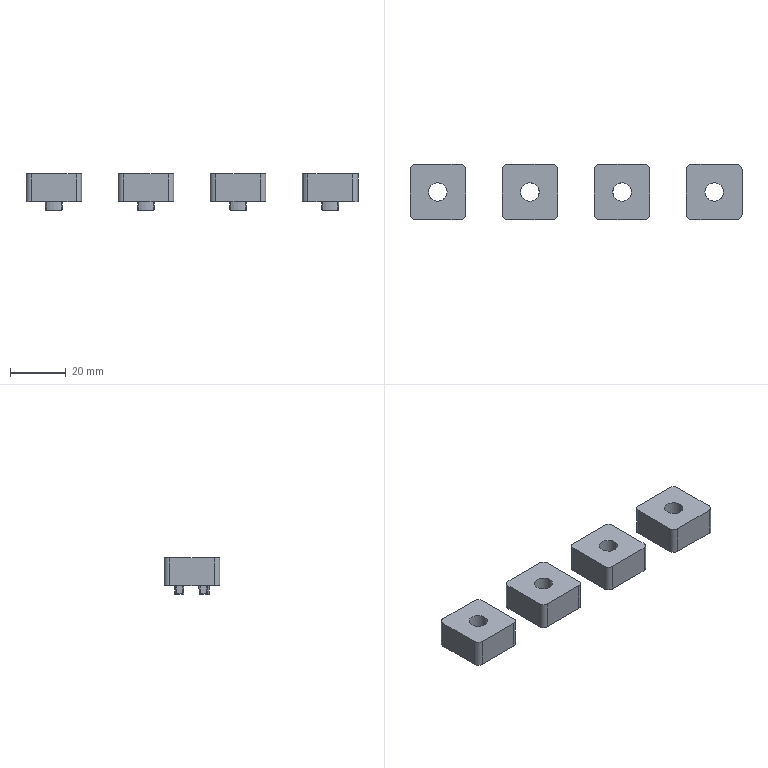NC program | NX | posted with a generic post | part box 118.91 x 19.91 x 13 mm
Lines 4009 to 4960 of 17620:
(FLOOR_WALL_1 , TOOL : D6)
N7992 T12 M6
N7994 G54
N7996 G17 G0 G90 X63.955 Y1.212 S9500 M3
N7998 G43 Z30. H12
N8000 Z0.92
N8002 G94 G1 Z-0.58 F1000.
N8004 X62.755 Y0.52
N8006 G3 X62.455 Y0. R0.6
N8008 G1 Y-8. F2500.
N8010 G2 X57.5 Y-12.955 R4.955
N8012 G1 X41.5
N8014 G2 X36.545 Y-8. R4.955
N8016 G1 Y8.
N8018 G2 X41.5 Y12.955 R4.955
N8020 G1 X45.778
N8022 Y9.355
N8024 G3 X45.124 Y9.068 R10.068
N8026 G1 X44.751 Y8.887
N8028 X44.592 Y8.783
N8030 X43.46 Y7.799
N8032 G3 X43.25 Y7.486 R0.72
N8034 G1 X42.72 Y5.917
N8036 G3 X42.682 Y5.687 R0.72
N8038 G1 X42.685 Y2.783
N8040 X42.766 Y1.87
N8042 G3 X42.861 Y1.573 R0.72
N8044 G1 X43.943 Y-0.291
N8046 G3 X44.32 Y-0.606 R0.72
N8048 G1 X44.45 Y-0.653
N8050 X44.411 Y-0.741
N8052 X43.725 Y-2.632
N8054 G3 X43.682 Y-2.878 R0.72
N8056 G1 Y-6.018
N8058 G3 X43.714 Y-6.231 R0.72
N8060 G1 X44.153 Y-7.65
N8062 G3 X44.321 Y-7.935 R0.72
N8064 G1 X45.313 Y-8.97
N8066 G3 X45.504 Y-9.112 R0.72
N8068 G1 X45.979 Y-9.355
N8070 X41.5
N8072 G2 X40.145 Y-8. R1.355
N8074 G1 Y8.
N8076 G2 X41.5 Y9.355 R1.355
N8078 G1 X45.778
N8080 Y12.955
N8082 X57.5
N8084 G2 X62.455 Y8. R4.955
N8086 G1 Y0.
N8088 X58.855
N8090 Y-8.
N8092 G2 X57.5 Y-9.355 R1.355
N8094 G1 X53.022
N8096 X54.029 Y-8.717
N8098 G3 X54.26 Y-8.481 R0.72
N8100 G1 X55.001 Y-7.255
N8102 G3 X55.089 Y-7.031 R0.72
N8104 G1 X55.303 Y-6.022
N8106 X55.318 Y-5.874
N8108 X55.317 Y-3.292
N8110 X55.272 Y-2.508
N8112 G3 X55.197 Y-2.228 R0.72
N8114 G1 X54.38 Y-0.593
N8116 X55.274 Y-0.074
N8118 G3 X55.589 Y0.303 R0.72
N8120 G1 X56.275 Y2.194
N8122 G3 X56.318 Y2.439 R0.72
N8124 G1 Y5.59
N8126 X56.293 Y5.778
N8128 X55.902 Y7.222
N8130 G3 X55.712 Y7.547 R0.72
N8132 G1 X54.529 Y8.71
N8134 G3 X54.337 Y8.845 R0.72
N8136 G1 X53.876 Y9.068
N8138 G3 X53.222 Y9.355 R10.068
N8140 G1 X52.956 Y8.686
N8142 G2 X53.563 Y8.419 R9.348
N8144 G1 X54.024 Y8.197
N8146 X55.207 Y7.034
N8148 X55.598 Y5.59
N8150 Y2.439
N8152 X54.912 Y0.549
N8154 X53.158 Y-0.47
N8156 X53.612 Y-0.668
N8158 X54.553 Y-2.55
N8160 X54.598 Y-3.334
N8162 Y-5.874
N8164 X54.385 Y-6.883
N8166 X53.644 Y-8.109
N8168 X52.39 Y-8.903
N8170 X51.937 Y-9.025
N8172 G2 X47.063 Y-9.025 R9.348
N8174 G1 X46.749 Y-8.94
N8176 X45.832 Y-8.471
N8178 X44.841 Y-7.437
N8180 X44.402 Y-6.018
N8182 Y-2.878
N8184 X45.088 Y-0.987
N8186 X46.008 Y-0.453
N8188 X44.566 Y0.071
N8190 X43.483 Y1.934
N8192 X43.402 Y2.847
N8194 Y5.687
N8196 X43.932 Y7.255
N8198 X45.064 Y8.239
N8200 X45.437 Y8.419
N8202 G2 X52.956 Y8.686 R9.348
N8204 G1 X53.222 Y9.355
N8206 X57.5
N8208 G2 X58.855 Y8. R1.355
N8210 G1 Y0.
N8212 G3 X59.155 Y-0.52 R0.6
N8214 G1 Z0.92
N8216 G0 X63.955 Y1.212 Z0.34
N8218 G1 Z-1.16 F1000.
N8220 X62.755 Y0.52
N8222 G3 X62.455 Y0. R0.6
N8224 G1 Y-8. F2500.
N8226 G2 X57.5 Y-12.955 R4.955
N8228 G1 X41.5
N8230 G2 X36.545 Y-8. R4.955
N8232 G1 Y8.
N8234 G2 X41.5 Y12.955 R4.955
N8236 G1 X45.778
N8238 Y9.355
N8240 G3 X45.124 Y9.068 R10.068
N8242 G1 X44.751 Y8.887
N8244 X44.592 Y8.783
N8246 X43.46 Y7.799
N8248 G3 X43.25 Y7.486 R0.72
N8250 G1 X42.72 Y5.917
N8252 G3 X42.682 Y5.687 R0.72
N8254 G1 X42.685 Y2.783
N8256 X42.766 Y1.87
N8258 G3 X42.861 Y1.573 R0.72
N8260 G1 X43.943 Y-0.291
N8262 G3 X44.32 Y-0.606 R0.72
N8264 G1 X44.45 Y-0.653
N8266 X44.411 Y-0.741
N8268 X43.725 Y-2.632
N8270 G3 X43.682 Y-2.878 R0.72
N8272 G1 Y-6.018
N8274 G3 X43.714 Y-6.231 R0.72
N8276 G1 X44.153 Y-7.65
N8278 G3 X44.321 Y-7.935 R0.72
N8280 G1 X45.313 Y-8.97
N8282 G3 X45.504 Y-9.112 R0.72
N8284 G1 X45.979 Y-9.355
N8286 X41.5
N8288 G2 X40.145 Y-8. R1.355
N8290 G1 Y8.
N8292 G2 X41.5 Y9.355 R1.355
N8294 G1 X45.778
N8296 Y12.955
N8298 X57.5
N8300 G2 X62.455 Y8. R4.955
N8302 G1 Y0.
N8304 X58.855
N8306 Y-8.
N8308 G2 X57.5 Y-9.355 R1.355
N8310 G1 X53.022
N8312 X54.029 Y-8.717
N8314 G3 X54.26 Y-8.481 R0.72
N8316 G1 X55.001 Y-7.255
N8318 G3 X55.089 Y-7.031 R0.72
N8320 G1 X55.303 Y-6.022
N8322 X55.318 Y-5.874
N8324 X55.317 Y-3.292
N8326 X55.272 Y-2.508
N8328 G3 X55.197 Y-2.228 R0.72
N8330 G1 X54.38 Y-0.593
N8332 X55.274 Y-0.074
N8334 G3 X55.589 Y0.303 R0.72
N8336 G1 X56.275 Y2.194
N8338 G3 X56.318 Y2.439 R0.72
N8340 G1 Y5.59
N8342 X56.293 Y5.778
N8344 X55.902 Y7.222
N8346 G3 X55.712 Y7.547 R0.72
N8348 G1 X54.529 Y8.71
N8350 G3 X54.337 Y8.845 R0.72
N8352 G1 X53.876 Y9.068
N8354 G3 X53.222 Y9.355 R10.068
N8356 G1 X52.956 Y8.686
N8358 G2 X53.563 Y8.419 R9.348
N8360 G1 X54.024 Y8.197
N8362 X55.207 Y7.034
N8364 X55.598 Y5.59
N8366 Y2.439
N8368 X54.912 Y0.549
N8370 X53.158 Y-0.47
N8372 X53.612 Y-0.668
N8374 X54.553 Y-2.55
N8376 X54.598 Y-3.334
N8378 Y-5.874
N8380 X54.385 Y-6.883
N8382 X53.644 Y-8.109
N8384 X52.39 Y-8.903
N8386 X51.937 Y-9.025
N8388 G2 X47.063 Y-9.025 R9.348
N8390 G1 X46.749 Y-8.94
N8392 X45.832 Y-8.471
N8394 X44.841 Y-7.437
N8396 X44.402 Y-6.018
N8398 Y-2.878
N8400 X45.088 Y-0.987
N8402 X46.008 Y-0.453
N8404 X44.566 Y0.071
N8406 X43.483 Y1.934
N8408 X43.402 Y2.847
N8410 Y5.687
N8412 X43.932 Y7.255
N8414 X45.064 Y8.239
N8416 X45.437 Y8.419
N8418 G2 X52.956 Y8.686 R9.348
N8420 G1 X53.222 Y9.355
N8422 X57.5
N8424 G2 X58.855 Y8. R1.355
N8426 G1 Y0.
N8428 G3 X59.155 Y-0.52 R0.6
N8430 G1 Z0.34
N8432 G0 X63.955 Y1.212 Z-0.24
N8434 G1 Z-1.74 F1000.
N8436 X62.755 Y0.52
N8438 G3 X62.455 Y0. R0.6
N8440 G1 Y-8. F2500.
N8442 G2 X57.5 Y-12.955 R4.955
N8444 G1 X41.5
N8446 G2 X36.545 Y-8. R4.955
N8448 G1 Y8.
N8450 G2 X41.5 Y12.955 R4.955
N8452 G1 X45.778
N8454 Y9.355
N8456 G3 X45.124 Y9.068 R10.068
N8458 G1 X44.751 Y8.887
N8460 X44.592 Y8.783
N8462 X43.46 Y7.799
N8464 G3 X43.25 Y7.486 R0.72
N8466 G1 X42.72 Y5.917
N8468 G3 X42.682 Y5.687 R0.72
N8470 G1 X42.685 Y2.783
N8472 X42.766 Y1.87
N8474 G3 X42.861 Y1.573 R0.72
N8476 G1 X43.943 Y-0.291
N8478 G3 X44.32 Y-0.606 R0.72
N8480 G1 X44.45 Y-0.653
N8482 X44.411 Y-0.741
N8484 X43.725 Y-2.632
N8486 G3 X43.682 Y-2.878 R0.72
N8488 G1 Y-6.018
N8490 G3 X43.714 Y-6.231 R0.72
N8492 G1 X44.153 Y-7.65
N8494 G3 X44.321 Y-7.935 R0.72
N8496 G1 X45.313 Y-8.97
N8498 G3 X45.504 Y-9.112 R0.72
N8500 G1 X45.979 Y-9.355
N8502 X41.5
N8504 G2 X40.145 Y-8. R1.355
N8506 G1 Y8.
N8508 G2 X41.5 Y9.355 R1.355
N8510 G1 X45.778
N8512 Y12.955
N8514 X57.5
N8516 G2 X62.455 Y8. R4.955
N8518 G1 Y0.
N8520 X58.855
N8522 Y-8.
N8524 G2 X57.5 Y-9.355 R1.355
N8526 G1 X53.022
N8528 X54.029 Y-8.717
N8530 G3 X54.26 Y-8.481 R0.72
N8532 G1 X55.001 Y-7.255
N8534 G3 X55.089 Y-7.031 R0.72
N8536 G1 X55.303 Y-6.022
N8538 X55.318 Y-5.874
N8540 X55.317 Y-3.292
N8542 X55.272 Y-2.508
N8544 G3 X55.197 Y-2.228 R0.72
N8546 G1 X54.38 Y-0.593
N8548 X55.274 Y-0.074
N8550 G3 X55.589 Y0.303 R0.72
N8552 G1 X56.275 Y2.194
N8554 G3 X56.318 Y2.439 R0.72
N8556 G1 Y5.59
N8558 X56.293 Y5.778
N8560 X55.902 Y7.222
N8562 G3 X55.712 Y7.547 R0.72
N8564 G1 X54.529 Y8.71
N8566 G3 X54.337 Y8.845 R0.72
N8568 G1 X53.876 Y9.068
N8570 G3 X53.222 Y9.355 R10.068
N8572 G1 X52.956 Y8.686
N8574 G2 X53.563 Y8.419 R9.348
N8576 G1 X54.024 Y8.197
N8578 X55.207 Y7.034
N8580 X55.598 Y5.59
N8582 Y2.439
N8584 X54.912 Y0.549
N8586 X53.158 Y-0.47
N8588 X53.612 Y-0.668
N8590 X54.553 Y-2.55
N8592 X54.598 Y-3.334
N8594 Y-5.874
N8596 X54.385 Y-6.883
N8598 X53.644 Y-8.109
N8600 X52.39 Y-8.903
N8602 X51.937 Y-9.025
N8604 G2 X47.063 Y-9.025 R9.348
N8606 G1 X46.749 Y-8.94
N8608 X45.832 Y-8.471
N8610 X44.841 Y-7.437
N8612 X44.402 Y-6.018
N8614 Y-2.878
N8616 X45.088 Y-0.987
N8618 X46.008 Y-0.453
N8620 X44.566 Y0.071
N8622 X43.483 Y1.934
N8624 X43.402 Y2.847
N8626 Y5.687
N8628 X43.932 Y7.255
N8630 X45.064 Y8.239
N8632 X45.437 Y8.419
N8634 G2 X52.956 Y8.686 R9.348
N8636 G1 X53.222 Y9.355
N8638 X57.5
N8640 G2 X58.855 Y8. R1.355
N8642 G1 Y0.
N8644 G3 X59.155 Y-0.52 R0.6
N8646 G1 Z-0.24
N8648 G0 X63.955 Y1.212 Z-0.82
N8650 G1 Z-2.32 F1000.
N8652 X62.755 Y0.52
N8654 G3 X62.455 Y0. R0.6
N8656 G1 Y-8. F2500.
N8658 G2 X57.5 Y-12.955 R4.955
N8660 G1 X41.5
N8662 G2 X36.545 Y-8. R4.955
N8664 G1 Y8.
N8666 G2 X41.5 Y12.955 R4.955
N8668 G1 X45.778
N8670 Y9.355
N8672 G3 X45.124 Y9.068 R10.068
N8674 G1 X44.751 Y8.887
N8676 X44.592 Y8.783
N8678 X43.46 Y7.799
N8680 G3 X43.25 Y7.486 R0.72
N8682 G1 X42.72 Y5.917
N8684 G3 X42.682 Y5.687 R0.72
N8686 G1 X42.685 Y2.783
N8688 X42.766 Y1.87
N8690 G3 X42.861 Y1.573 R0.72
N8692 G1 X43.943 Y-0.291
N8694 G3 X44.32 Y-0.606 R0.72
N8696 G1 X44.45 Y-0.653
N8698 X44.411 Y-0.741
N8700 X43.725 Y-2.632
N8702 G3 X43.682 Y-2.878 R0.72
N8704 G1 Y-6.018
N8706 G3 X43.714 Y-6.231 R0.72
N8708 G1 X44.153 Y-7.65
N8710 G3 X44.321 Y-7.935 R0.72
N8712 G1 X45.313 Y-8.97
N8714 G3 X45.504 Y-9.112 R0.72
N8716 G1 X45.979 Y-9.355
N8718 X41.5
N8720 G2 X40.145 Y-8. R1.355
N8722 G1 Y8.
N8724 G2 X41.5 Y9.355 R1.355
N8726 G1 X45.778
N8728 Y12.955
N8730 X57.5
N8732 G2 X62.455 Y8. R4.955
N8734 G1 Y0.
N8736 X58.855
N8738 Y-8.
N8740 G2 X57.5 Y-9.355 R1.355
N8742 G1 X53.022
N8744 X54.029 Y-8.717
N8746 G3 X54.26 Y-8.481 R0.72
N8748 G1 X55.001 Y-7.255
N8750 G3 X55.089 Y-7.031 R0.72
N8752 G1 X55.303 Y-6.022
N8754 X55.318 Y-5.874
N8756 X55.317 Y-3.292
N8758 X55.272 Y-2.508
N8760 G3 X55.197 Y-2.228 R0.72
N8762 G1 X54.38 Y-0.593
N8764 X55.274 Y-0.074
N8766 G3 X55.589 Y0.303 R0.72
N8768 G1 X56.275 Y2.194
N8770 G3 X56.318 Y2.439 R0.72
N8772 G1 Y5.59
N8774 X56.293 Y5.778
N8776 X55.902 Y7.222
N8778 G3 X55.712 Y7.547 R0.72
N8780 G1 X54.529 Y8.71
N8782 G3 X54.337 Y8.845 R0.72
N8784 G1 X53.876 Y9.068
N8786 G3 X53.222 Y9.355 R10.068
N8788 G1 X52.956 Y8.686
N8790 G2 X53.563 Y8.419 R9.348
N8792 G1 X54.024 Y8.197
N8794 X55.207 Y7.034
N8796 X55.598 Y5.59
N8798 Y2.439
N8800 X54.912 Y0.549
N8802 X53.158 Y-0.47
N8804 X53.612 Y-0.668
N8806 X54.553 Y-2.55
N8808 X54.598 Y-3.334
N8810 Y-5.874
N8812 X54.385 Y-6.883
N8814 X53.644 Y-8.109
N8816 X52.39 Y-8.903
N8818 X51.937 Y-9.025
N8820 G2 X47.063 Y-9.025 R9.348
N8822 G1 X46.749 Y-8.94
N8824 X45.832 Y-8.471
N8826 X44.841 Y-7.437
N8828 X44.402 Y-6.018
N8830 Y-2.878
N8832 X45.088 Y-0.987
N8834 X46.008 Y-0.453
N8836 X44.566 Y0.071
N8838 X43.483 Y1.934
N8840 X43.402 Y2.847
N8842 Y5.687
N8844 X43.932 Y7.255
N8846 X45.064 Y8.239
N8848 X45.437 Y8.419
N8850 G2 X52.956 Y8.686 R9.348
N8852 G1 X53.222 Y9.355
N8854 X57.5
N8856 G2 X58.855 Y8. R1.355
N8858 G1 Y0.
N8860 G3 X59.155 Y-0.52 R0.6
N8862 G1 Z-0.82
N8864 G0 X63.955 Y1.212 Z-1.4
N8866 G1 Z-2.9 F1000.
N8868 X62.755 Y0.52
N8870 G3 X62.455 Y0. R0.6
N8872 G1 Y-8. F2500.
N8874 G2 X57.5 Y-12.955 R4.955
N8876 G1 X41.5
N8878 G2 X36.545 Y-8. R4.955
N8880 G1 Y8.
N8882 G2 X41.5 Y12.955 R4.955
N8884 G1 X45.778
N8886 Y9.355
N8888 G3 X45.124 Y9.068 R10.068
N8890 G1 X44.751 Y8.887
N8892 X44.592 Y8.783
N8894 X43.46 Y7.799
N8896 G3 X43.25 Y7.486 R0.72
N8898 G1 X42.72 Y5.917
N8900 G3 X42.682 Y5.687 R0.72
N8902 G1 X42.685 Y2.783
N8904 X42.766 Y1.87
N8906 G3 X42.861 Y1.573 R0.72
N8908 G1 X43.943 Y-0.291
N8910 G3 X44.32 Y-0.606 R0.72
N8912 G1 X44.45 Y-0.653
N8914 X44.411 Y-0.741
N8916 X43.725 Y-2.632
N8918 G3 X43.682 Y-2.878 R0.72
N8920 G1 Y-6.018
N8922 G3 X43.714 Y-6.231 R0.72
N8924 G1 X44.153 Y-7.65
N8926 G3 X44.321 Y-7.935 R0.72
N8928 G1 X45.313 Y-8.97
N8930 G3 X45.504 Y-9.112 R0.72
N8932 G1 X45.979 Y-9.355
N8934 X41.5
N8936 G2 X40.145 Y-8. R1.355
N8938 G1 Y8.
N8940 G2 X41.5 Y9.355 R1.355
N8942 G1 X45.778
N8944 Y12.955
N8946 X57.5
N8948 G2 X62.455 Y8. R4.955
N8950 G1 Y0.
N8952 X58.855
N8954 Y-8.
N8956 G2 X57.5 Y-9.355 R1.355
N8958 G1 X53.022
N8960 X54.029 Y-8.717
N8962 G3 X54.26 Y-8.481 R0.72
N8964 G1 X55.001 Y-7.255
N8966 G3 X55.089 Y-7.031 R0.72
N8968 G1 X55.303 Y-6.022
N8970 X55.318 Y-5.874
N8972 X55.317 Y-3.292
N8974 X55.272 Y-2.508
N8976 G3 X55.197 Y-2.228 R0.72
N8978 G1 X54.38 Y-0.593
N8980 X55.274 Y-0.074
N8982 G3 X55.589 Y0.303 R0.72
N8984 G1 X56.275 Y2.194
N8986 G3 X56.318 Y2.439 R0.72
N8988 G1 Y5.59
N8990 X56.293 Y5.778
N8992 X55.902 Y7.222
N8994 G3 X55.712 Y7.547 R0.72
N8996 G1 X54.529 Y8.71
N8998 G3 X54.337 Y8.845 R0.72
N9000 G1 X53.876 Y9.068
N9002 G3 X53.222 Y9.355 R10.068
N9004 G1 X52.956 Y8.686
N9006 G2 X53.563 Y8.419 R9.348
N9008 G1 X54.024 Y8.197
N9010 X55.207 Y7.034
N9012 X55.598 Y5.59
N9014 Y2.439
N9016 X54.912 Y0.549
N9018 X53.158 Y-0.47
N9020 X53.612 Y-0.668
N9022 X54.553 Y-2.55
N9024 X54.598 Y-3.334
N9026 Y-5.874
N9028 X54.385 Y-6.883
N9030 X53.644 Y-8.109
N9032 X52.39 Y-8.903
N9034 X51.937 Y-9.025
N9036 G2 X47.063 Y-9.025 R9.348
N9038 G1 X46.749 Y-8.94
N9040 X45.832 Y-8.471
N9042 X44.841 Y-7.437
N9044 X44.402 Y-6.018
N9046 Y-2.878
N9048 X45.088 Y-0.987
N9050 X46.008 Y-0.453
N9052 X44.566 Y0.071
N9054 X43.483 Y1.934
N9056 X43.402 Y2.847
N9058 Y5.687
N9060 X43.932 Y7.255
N9062 X45.064 Y8.239
N9064 X45.437 Y8.419
N9066 G2 X52.956 Y8.686 R9.348
N9068 G1 X53.222 Y9.355
N9070 X57.5
N9072 G2 X58.855 Y8. R1.355
N9074 G1 Y0.
N9076 G3 X59.155 Y-0.52 R0.6
N9078 G1 Z-1.4
N9080 G0 Z30.
N9082 X49.153 Y-0.044
N9084 Z1.5
N9086 G1 X49.148 Y-0.042 Z1.499 F1000.
N9088 X49.2 Y0.003 Z1.48
N9090 X49.148 Y-0.042 Z1.462
N9092 X49.209 Y-0.074 Z1.443
N9094 X49.148 Y-0.042 Z1.425
N9096 X49.2 Y0.003 Z1.407
N9098 X49.148 Y-0.042 Z1.388
N9100 X49.209 Y-0.074 Z1.37
N9102 X49.148 Y-0.042 Z1.352
N9104 X49.2 Y0.003 Z1.333
N9106 X49.148 Y-0.042 Z1.315
N9108 X49.209 Y-0.074 Z1.296
N9110 X49.148 Y-0.042 Z1.278
N9112 X49.2 Y0.003 Z1.26
N9114 X49.148 Y-0.042 Z1.241
N9116 X49.209 Y-0.074 Z1.223
N9118 X49.148 Y-0.042 Z1.204
N9120 X49.2 Y0.003 Z1.186
N9122 X49.148 Y-0.042 Z1.168
N9124 X49.209 Y-0.074 Z1.149
N9126 X49.148 Y-0.042 Z1.131
N9128 X49.2 Y0.003 Z1.112
N9130 X49.148 Y-0.042 Z1.094
N9132 X49.209 Y-0.074 Z1.076
N9134 X49.148 Y-0.042 Z1.057
N9136 X49.2 Y0.003 Z1.039
N9138 X49.148 Y-0.042 Z1.02
N9140 X49.209 Y-0.074 Z1.002
N9142 X49.148 Y-0.042 Z0.984
N9144 X49.2 Y0.003 Z0.965
N9146 X49.148 Y-0.042 Z0.947
N9148 X49.209 Y-0.074 Z0.928
N9150 X49.148 Y-0.042 Z0.91
N9152 X49.2 Y0.003 Z0.892
N9154 X49.148 Y-0.042 Z0.873
N9156 X49.209 Y-0.074 Z0.855
N9158 X49.148 Y-0.042 Z0.836
N9160 X49.2 Y0.003 Z0.818
N9162 X49.148 Y-0.042 Z0.8
N9164 X49.209 Y-0.074 Z0.781
N9166 X49.148 Y-0.042 Z0.763
N9168 X49.2 Y0.003 Z0.744
N9170 X49.148 Y-0.042 Z0.726
N9172 X49.209 Y-0.074 Z0.708
N9174 X49.148 Y-0.042 Z0.689
N9176 X49.2 Y0.003 Z0.671
N9178 X49.148 Y-0.042 Z0.652
N9180 X49.209 Y-0.074 Z0.634
N9182 X49.148 Y-0.042 Z0.616
N9184 X49.2 Y0.003 Z0.597
N9186 X49.148 Y-0.042 Z0.579
N9188 X49.209 Y-0.074 Z0.561
N9190 X49.148 Y-0.042 Z0.542
N9192 X49.2 Y0.003 Z0.524
N9194 X49.148 Y-0.042 Z0.505
N9196 X49.209 Y-0.074 Z0.487
N9198 X49.148 Y-0.042 Z0.469
N9200 X49.2 Y0.003 Z0.45
N9202 X49.148 Y-0.042 Z0.432
N9204 X49.209 Y-0.074 Z0.413
N9206 X49.148 Y-0.042 Z0.395
N9208 X49.2 Y0.003 Z0.377
N9210 X49.148 Y-0.042 Z0.358
N9212 X49.209 Y-0.074 Z0.34
N9214 X49.148 Y-0.042 Z0.321
N9216 X49.2 Y0.003 Z0.303
N9218 X49.148 Y-0.042 Z0.285
N9220 X49.209 Y-0.074 Z0.266
N9222 X49.148 Y-0.042 Z0.248
N9224 X49.2 Y0.003 Z0.229
N9226 X49.148 Y-0.042 Z0.211
N9228 X49.209 Y-0.074 Z0.193
N9230 X49.148 Y-0.042 Z0.174
N9232 X49.2 Y0.003 Z0.156
N9234 X49.148 Y-0.042 Z0.137
N9236 X49.209 Y-0.074 Z0.119
N9238 X49.148 Y-0.042 Z0.101
N9240 X49.2 Y0.003 Z0.082
N9242 X49.148 Y-0.042 Z0.064
N9244 X49.209 Y-0.074 Z0.045
N9246 X49.148 Y-0.042 Z0.027
N9248 X49.2 Y0.003 Z0.009
N9250 X49.148 Y-0.042 Z-0.01
N9252 X49.209 Y-0.074 Z-0.028
N9254 X49.148 Y-0.042 Z-0.047
N9256 X49.2 Y0.003 Z-0.065
N9258 X49.148 Y-0.042 Z-0.083
N9260 X49.209 Y-0.074 Z-0.102
N9262 X49.148 Y-0.042 Z-0.12
N9264 X49.2 Y0.003 Z-0.139
N9266 X49.148 Y-0.042 Z-0.157
N9268 X49.209 Y-0.074 Z-0.175
N9270 X49.148 Y-0.042 Z-0.194
N9272 X49.2 Y0.003 Z-0.212
N9274 X49.148 Y-0.042 Z-0.23
N9276 X49.209 Y-0.074 Z-0.249
N9278 X49.148 Y-0.042 Z-0.267
N9280 X49.2 Y0.003 Z-0.286
N9282 X49.148 Y-0.042 Z-0.304
N9284 X49.209 Y-0.074 Z-0.322
N9286 X49.148 Y-0.042 Z-0.341
N9288 X49.2 Y0.003 Z-0.359
N9290 X49.148 Y-0.042 Z-0.378
N9292 X49.209 Y-0.074 Z-0.396
N9294 X49.148 Y-0.042 Z-0.414
N9296 X49.2 Y0.003 Z-0.433
N9298 X49.148 Y-0.042 Z-0.451
N9300 X49.209 Y-0.074 Z-0.47
N9302 X49.148 Y-0.042 Z-0.488
N9304 X49.2 Y0.003 Z-0.506
N9306 X49.148 Y-0.042 Z-0.525
N9308 X49.209 Y-0.074 Z-0.543
N9310 X49.148 Y-0.042 Z-0.562
N9312 X49.2 Y0.003 Z-0.58
N9314 X49.148 Y-0.042 F2500.
N9316 X49.209 Y-0.074
N9318 Z0.92
N9320 G0 X49.153 Y-0.044
N9322 G1 X49.148 Y-0.042 Z0.919 F1000.
N9324 X49.2 Y0.003 Z0.9
N9326 X49.148 Y-0.042 Z0.882
N9328 X49.209 Y-0.074 Z0.863
N9330 X49.148 Y-0.042 Z0.845
N9332 X49.2 Y0.003 Z0.827
N9334 X49.148 Y-0.042 Z0.808
N9336 X49.209 Y-0.074 Z0.79
N9338 X49.148 Y-0.042 Z0.772
N9340 X49.2 Y0.003 Z0.753
N9342 X49.148 Y-0.042 Z0.735
N9344 X49.209 Y-0.074 Z0.716
N9346 X49.148 Y-0.042 Z0.698
N9348 X49.2 Y0.003 Z0.68
N9350 X49.148 Y-0.042 Z0.661
N9352 X49.209 Y-0.074 Z0.643
N9354 X49.148 Y-0.042 Z0.624
N9356 X49.2 Y0.003 Z0.606
N9358 X49.148 Y-0.042 Z0.588
N9360 X49.209 Y-0.074 Z0.569
N9362 X49.148 Y-0.042 Z0.551
N9364 X49.2 Y0.003 Z0.532
N9366 X49.148 Y-0.042 Z0.514
N9368 X49.209 Y-0.074 Z0.496
N9370 X49.148 Y-0.042 Z0.477
N9372 X49.2 Y0.003 Z0.459
N9374 X49.148 Y-0.042 Z0.44
N9376 X49.209 Y-0.074 Z0.422
N9378 X49.148 Y-0.042 Z0.404
N9380 X49.2 Y0.003 Z0.385
N9382 X49.148 Y-0.042 Z0.367
N9384 X49.209 Y-0.074 Z0.348
N9386 X49.148 Y-0.042 Z0.33
N9388 X49.2 Y0.003 Z0.312
N9390 X49.148 Y-0.042 Z0.293
N9392 X49.209 Y-0.074 Z0.275
N9394 X49.148 Y-0.042 Z0.256
N9396 X49.2 Y0.003 Z0.238
N9398 X49.148 Y-0.042 Z0.22
N9400 X49.209 Y-0.074 Z0.201
N9402 X49.148 Y-0.042 Z0.183
N9404 X49.2 Y0.003 Z0.164
N9406 X49.148 Y-0.042 Z0.146
N9408 X49.209 Y-0.074 Z0.128
N9410 X49.148 Y-0.042 Z0.109
N9412 X49.2 Y0.003 Z0.091
N9414 X49.148 Y-0.042 Z0.072
N9416 X49.209 Y-0.074 Z0.054
N9418 X49.148 Y-0.042 Z0.036
N9420 X49.2 Y0.003 Z0.017
N9422 X49.148 Y-0.042 Z-0.001
N9424 X49.209 Y-0.074 Z-0.019
N9426 X49.148 Y-0.042 Z-0.038
N9428 X49.2 Y0.003 Z-0.056
N9430 X49.148 Y-0.042 Z-0.075
N9432 X49.209 Y-0.074 Z-0.093
N9434 X49.148 Y-0.042 Z-0.111
N9436 X49.2 Y0.003 Z-0.13
N9438 X49.148 Y-0.042 Z-0.148
N9440 X49.209 Y-0.074 Z-0.167
N9442 X49.148 Y-0.042 Z-0.185
N9444 X49.2 Y0.003 Z-0.203
N9446 X49.148 Y-0.042 Z-0.222
N9448 X49.209 Y-0.074 Z-0.24
N9450 X49.148 Y-0.042 Z-0.259
N9452 X49.2 Y0.003 Z-0.277
N9454 X49.148 Y-0.042 Z-0.295
N9456 X49.209 Y-0.074 Z-0.314
N9458 X49.148 Y-0.042 Z-0.332
N9460 X49.2 Y0.003 Z-0.351
N9462 X49.148 Y-0.042 Z-0.369
N9464 X49.209 Y-0.074 Z-0.387
N9466 X49.148 Y-0.042 Z-0.406
N9468 X49.2 Y0.003 Z-0.424
N9470 X49.148 Y-0.042 Z-0.443
N9472 X49.209 Y-0.074 Z-0.461
N9474 X49.148 Y-0.042 Z-0.479
N9476 X49.2 Y0.003 Z-0.498
N9478 X49.148 Y-0.042 Z-0.516
N9480 X49.209 Y-0.074 Z-0.535
N9482 X49.148 Y-0.042 Z-0.553
N9484 X49.2 Y0.003 Z-0.571
N9486 X49.148 Y-0.042 Z-0.59
N9488 X49.209 Y-0.074 Z-0.608
N9490 X49.148 Y-0.042 Z-0.627
N9492 X49.2 Y0.003 Z-0.645
N9494 X49.148 Y-0.042 Z-0.663
N9496 X49.209 Y-0.074 Z-0.682
N9498 X49.148 Y-0.042 Z-0.7
N9500 X49.2 Y0.003 Z-0.719
N9502 X49.148 Y-0.042 Z-0.737
N9504 X49.209 Y-0.074 Z-0.755
N9506 X49.148 Y-0.042 Z-0.774
N9508 X49.2 Y0.003 Z-0.792
N9510 X49.148 Y-0.042 Z-0.81
N9512 X49.209 Y-0.074 Z-0.829
N9514 X49.148 Y-0.042 Z-0.847
N9516 X49.2 Y0.003 Z-0.866
N9518 X49.148 Y-0.042 Z-0.884
N9520 X49.209 Y-0.074 Z-0.902
N9522 X49.148 Y-0.042 Z-0.921
N9524 X49.2 Y0.003 Z-0.939
N9526 X49.148 Y-0.042 Z-0.958
N9528 X49.209 Y-0.074 Z-0.976
N9530 X49.148 Y-0.042 Z-0.994
N9532 X49.2 Y0.003 Z-1.013
N9534 X49.148 Y-0.042 Z-1.031
N9536 X49.209 Y-0.074 Z-1.05
N9538 X49.148 Y-0.042 Z-1.068
N9540 X49.2 Y0.003 Z-1.086
N9542 X49.148 Y-0.042 Z-1.105
N9544 X49.209 Y-0.074 Z-1.123
N9546 X49.148 Y-0.042 Z-1.142
N9548 X49.2 Y0.003 Z-1.16
N9550 X49.148 Y-0.042 F2500.
N9552 X49.209 Y-0.074
N9554 Z0.34
N9556 G0 X49.153 Y-0.044
N9558 G1 X49.148 Y-0.042 Z0.339 F1000.
N9560 X49.2 Y0.003 Z0.32
N9562 X49.148 Y-0.042 Z0.302
N9564 X49.209 Y-0.074 Z0.283
N9566 X49.148 Y-0.042 Z0.265
N9568 X49.2 Y0.003 Z0.247
N9570 X49.148 Y-0.042 Z0.228
N9572 X49.209 Y-0.074 Z0.21
N9574 X49.148 Y-0.042 Z0.192
N9576 X49.2 Y0.003 Z0.173
N9578 X49.148 Y-0.042 Z0.155
N9580 X49.209 Y-0.074 Z0.136
N9582 X49.148 Y-0.042 Z0.118
N9584 X49.2 Y0.003 Z0.1
N9586 X49.148 Y-0.042 Z0.081
N9588 X49.209 Y-0.074 Z0.063
N9590 X49.148 Y-0.042 Z0.044
N9592 X49.2 Y0.003 Z0.026
N9594 X49.148 Y-0.042 Z0.008
N9596 X49.209 Y-0.074 Z-0.011
N9598 X49.148 Y-0.042 Z-0.029
N9600 X49.2 Y0.003 Z-0.048
N9602 X49.148 Y-0.042 Z-0.066
N9604 X49.209 Y-0.074 Z-0.084
N9606 X49.148 Y-0.042 Z-0.103
N9608 X49.2 Y0.003 Z-0.121
N9610 X49.148 Y-0.042 Z-0.14
N9612 X49.209 Y-0.074 Z-0.158
N9614 X49.148 Y-0.042 Z-0.176
N9616 X49.2 Y0.003 Z-0.195
N9618 X49.148 Y-0.042 Z-0.213
N9620 X49.209 Y-0.074 Z-0.232
N9622 X49.148 Y-0.042 Z-0.25
N9624 X49.2 Y0.003 Z-0.268
N9626 X49.148 Y-0.042 Z-0.287
N9628 X49.209 Y-0.074 Z-0.305
N9630 X49.148 Y-0.042 Z-0.324
N9632 X49.2 Y0.003 Z-0.342
N9634 X49.148 Y-0.042 Z-0.36
N9636 X49.209 Y-0.074 Z-0.379
N9638 X49.148 Y-0.042 Z-0.397
N9640 X49.2 Y0.003 Z-0.416
N9642 X49.148 Y-0.042 Z-0.434
N9644 X49.209 Y-0.074 Z-0.452
N9646 X49.148 Y-0.042 Z-0.471
N9648 X49.2 Y0.003 Z-0.489
N9650 X49.148 Y-0.042 Z-0.508
N9652 X49.209 Y-0.074 Z-0.526
N9654 X49.148 Y-0.042 Z-0.544
N9656 X49.2 Y0.003 Z-0.563
N9658 X49.148 Y-0.042 Z-0.581
N9660 X49.209 Y-0.074 Z-0.599
N9662 X49.148 Y-0.042 Z-0.618
N9664 X49.2 Y0.003 Z-0.636
N9666 X49.148 Y-0.042 Z-0.655
N9668 X49.209 Y-0.074 Z-0.673
N9670 X49.148 Y-0.042 Z-0.691
N9672 X49.2 Y0.003 Z-0.71
N9674 X49.148 Y-0.042 Z-0.728
N9676 X49.209 Y-0.074 Z-0.747
N9678 X49.148 Y-0.042 Z-0.765
N9680 X49.2 Y0.003 Z-0.783
N9682 X49.148 Y-0.042 Z-0.802
N9684 X49.209 Y-0.074 Z-0.82
N9686 X49.148 Y-0.042 Z-0.839
N9688 X49.2 Y0.003 Z-0.857
N9690 X49.148 Y-0.042 Z-0.875
N9692 X49.209 Y-0.074 Z-0.894
N9694 X49.148 Y-0.042 Z-0.912
N9696 X49.2 Y0.003 Z-0.931
N9698 X49.148 Y-0.042 Z-0.949
N9700 X49.209 Y-0.074 Z-0.967
N9702 X49.148 Y-0.042 Z-0.986
N9704 X49.2 Y0.003 Z-1.004
N9706 X49.148 Y-0.042 Z-1.023
N9708 X49.209 Y-0.074 Z-1.041
N9710 X49.148 Y-0.042 Z-1.059
N9712 X49.2 Y0.003 Z-1.078
N9714 X49.148 Y-0.042 Z-1.096
N9716 X49.209 Y-0.074 Z-1.115
N9718 X49.148 Y-0.042 Z-1.133
N9720 X49.2 Y0.003 Z-1.151
N9722 X49.148 Y-0.042 Z-1.17
N9724 X49.209 Y-0.074 Z-1.188
N9726 X49.148 Y-0.042 Z-1.207
N9728 X49.2 Y0.003 Z-1.225
N9730 X49.148 Y-0.042 Z-1.243
N9732 X49.209 Y-0.074 Z-1.262
N9734 X49.148 Y-0.042 Z-1.28
N9736 X49.2 Y0.003 Z-1.299
N9738 X49.148 Y-0.042 Z-1.317
N9740 X49.209 Y-0.074 Z-1.335
N9742 X49.148 Y-0.042 Z-1.354
N9744 X49.2 Y0.003 Z-1.372
N9746 X49.148 Y-0.042 Z-1.39
N9748 X49.209 Y-0.074 Z-1.409
N9750 X49.148 Y-0.042 Z-1.427
N9752 X49.2 Y0.003 Z-1.446
N9754 X49.148 Y-0.042 Z-1.464
N9756 X49.209 Y-0.074 Z-1.482
N9758 X49.148 Y-0.042 Z-1.501
N9760 X49.2 Y0.003 Z-1.519
N9762 X49.148 Y-0.042 Z-1.538
N9764 X49.209 Y-0.074 Z-1.556
N9766 X49.148 Y-0.042 Z-1.574
N9768 X49.2 Y0.003 Z-1.593
N9770 X49.148 Y-0.042 Z-1.611
N9772 X49.209 Y-0.074 Z-1.63
N9774 X49.148 Y-0.042 Z-1.648
N9776 X49.2 Y0.003 Z-1.666
N9778 X49.148 Y-0.042 Z-1.685
N9780 X49.209 Y-0.074 Z-1.703
N9782 X49.148 Y-0.042 Z-1.722
N9784 X49.2 Y0.003 Z-1.74
N9786 X49.148 Y-0.042 F2500.
N9788 X49.209 Y-0.074
N9790 Z-0.24
N9792 G0 X49.153 Y-0.044
N9794 G1 X49.148 Y-0.042 Z-0.241 F1000.
N9796 X49.2 Y0.003 Z-0.26
N9798 X49.148 Y-0.042 Z-0.278
N9800 X49.209 Y-0.074 Z-0.297
N9802 X49.148 Y-0.042 Z-0.315
N9804 X49.2 Y0.003 Z-0.333
N9806 X49.148 Y-0.042 Z-0.352
N9808 X49.209 Y-0.074 Z-0.37
N9810 X49.148 Y-0.042 Z-0.388
N9812 X49.2 Y0.003 Z-0.407
N9814 X49.148 Y-0.042 Z-0.425
N9816 X49.209 Y-0.074 Z-0.444
N9818 X49.148 Y-0.042 Z-0.462
N9820 X49.2 Y0.003 Z-0.48
N9822 X49.148 Y-0.042 Z-0.499
N9824 X49.209 Y-0.074 Z-0.517
N9826 X49.148 Y-0.042 Z-0.536
N9828 X49.2 Y0.003 Z-0.554
N9830 X49.148 Y-0.042 Z-0.572
N9832 X49.209 Y-0.074 Z-0.591
N9834 X49.148 Y-0.042 Z-0.609
N9836 X49.2 Y0.003 Z-0.628
N9838 X49.148 Y-0.042 Z-0.646
N9840 X49.209 Y-0.074 Z-0.664
N9842 X49.148 Y-0.042 Z-0.683
N9844 X49.2 Y0.003 Z-0.701
N9846 X49.148 Y-0.042 Z-0.72
N9848 X49.209 Y-0.074 Z-0.738
N9850 X49.148 Y-0.042 Z-0.756
N9852 X49.2 Y0.003 Z-0.775
N9854 X49.148 Y-0.042 Z-0.793
N9856 X49.209 Y-0.074 Z-0.812
N9858 X49.148 Y-0.042 Z-0.83
N9860 X49.2 Y0.003 Z-0.848
N9862 X49.148 Y-0.042 Z-0.867
N9864 X49.209 Y-0.074 Z-0.885
N9866 X49.148 Y-0.042 Z-0.904
N9868 X49.2 Y0.003 Z-0.922
N9870 X49.148 Y-0.042 Z-0.94
N9872 X49.209 Y-0.074 Z-0.959
N9874 X49.148 Y-0.042 Z-0.977
N9876 X49.2 Y0.003 Z-0.996
N9878 X49.148 Y-0.042 Z-1.014
N9880 X49.209 Y-0.074 Z-1.032
N9882 X49.148 Y-0.042 Z-1.051
N9884 X49.2 Y0.003 Z-1.069
N9886 X49.148 Y-0.042 Z-1.088
N9888 X49.209 Y-0.074 Z-1.106